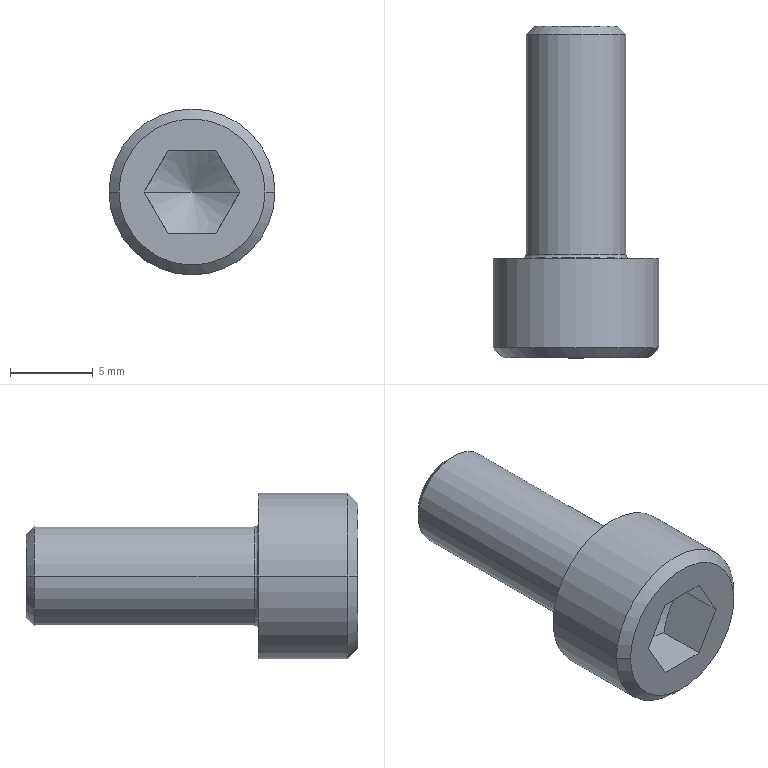Part | Creo | 1 solid | 23 faces | box 10 x 20 x 10 mm | volume 780.586 mm3 | plane 9 | cone 6 | cylinder 4 | torus 4 | commonest cylinder face diameters 6 x2 10 x2
STEP:
#1=CARTESIAN_POINT('',(0.,0.,0.));
#2=DIRECTION('',(0.,0.,1.));
#3=DIRECTION('',(1.,0.,0.));
#4=AXIS2_PLACEMENT_3D('',#1,#2,#3);
#5=CARTESIAN_POINT('',(-46.437,-246.,-26.767));
#6=VERTEX_POINT('',#5);
#7=CARTESIAN_POINT('',(-44.993,-246.,-29.267));
#8=VERTEX_POINT('',#7);
#9=CARTESIAN_POINT('',(-46.437,-246.,-26.767));
#10=CARTESIAN_POINT('',(-46.401,-245.979,-26.83));
#11=CARTESIAN_POINT('',(-46.329,-245.94,-26.953));
#12=CARTESIAN_POINT('',(-46.226,-245.891,-27.132));
#13=CARTESIAN_POINT('',(-46.124,-245.851,-27.308));
#14=CARTESIAN_POINT('',(-46.024,-245.819,-27.483));
#15=CARTESIAN_POINT('',(-45.922,-245.795,-27.659));
#16=CARTESIAN_POINT('',(-45.819,-245.78,-27.837));
#17=CARTESIAN_POINT('',(-45.715,-245.775,-28.017));
#18=CARTESIAN_POINT('',(-45.611,-245.78,-28.197));
#19=CARTESIAN_POINT('',(-45.508,-245.795,-28.375));
#20=CARTESIAN_POINT('',(-45.407,-245.819,-28.551));
#21=CARTESIAN_POINT('',(-45.306,-245.851,-28.726));
#22=CARTESIAN_POINT('',(-45.204,-245.891,-28.902));
#23=CARTESIAN_POINT('',(-45.101,-245.94,-29.081));
#24=CARTESIAN_POINT('',(-45.03,-245.979,-29.204));
#25=CARTESIAN_POINT('',(-44.993,-246.,-29.267));
#26=B_SPLINE_CURVE_WITH_KNOTS('',3,(#9,#10,#11,#12,#13,#14,#15,#16,#17,#18,#19,#20,#21,#22,#23,#24,#25),.UNSPECIFIED.,.F.,.F.,(4,1,1,1,1,1,1,1,1,1,1,1,1,1,4),(0.,0.07143,0.1429,0.2143,0.2857,0.3571,0.4286,0.5,0.5714,0.6429,0.7143,0.7857,0.8571,0.9286,1.),.UNSPECIFIED.);
#27=EDGE_CURVE('',#6,#8,#26,.T.);
#28=ORIENTED_EDGE('',*,*,#27,.F.);
#29=CARTESIAN_POINT('',(-43.55,-244.333,-26.767));
#30=VERTEX_POINT('',#29);
#31=CARTESIAN_POINT('',(-43.55,-244.333,-26.767));
#32=DIRECTION('',(-0.866,-0.5,0.));
#33=VECTOR('',#32,3.333);
#34=LINE('',#31,#33);
#35=EDGE_CURVE('',#30,#6,#34,.T.);
#36=ORIENTED_EDGE('',*,*,#35,.F.);
#37=CARTESIAN_POINT('',(-40.663,-246.,-26.767));
#38=VERTEX_POINT('',#37);
#39=CARTESIAN_POINT('',(-43.55,-244.333,-26.767));
#40=DIRECTION('',(0.866,-0.5,0.));
#41=VECTOR('',#40,3.333);
#42=LINE('',#39,#41);
#43=EDGE_CURVE('',#30,#38,#42,.T.);
#44=ORIENTED_EDGE('',*,*,#43,.T.);
#45=CARTESIAN_POINT('',(-42.107,-246.,-29.267));
#46=VERTEX_POINT('',#45);
#47=CARTESIAN_POINT('',(-42.107,-246.,-29.267));
#48=CARTESIAN_POINT('',(-42.07,-245.979,-29.204));
#49=CARTESIAN_POINT('',(-41.999,-245.94,-29.081));
#50=CARTESIAN_POINT('',(-41.896,-245.891,-28.902));
#51=CARTESIAN_POINT('',(-41.794,-245.851,-28.726));
#52=CARTESIAN_POINT('',(-41.693,-245.819,-28.551));
#53=CARTESIAN_POINT('',(-41.592,-245.795,-28.375));
#54=CARTESIAN_POINT('',(-41.489,-245.78,-28.197));
#55=CARTESIAN_POINT('',(-41.385,-245.775,-28.017));
#56=CARTESIAN_POINT('',(-41.281,-245.78,-27.837));
#57=CARTESIAN_POINT('',(-41.178,-245.795,-27.659));
#58=CARTESIAN_POINT('',(-41.076,-245.819,-27.483));
#59=CARTESIAN_POINT('',(-40.976,-245.851,-27.308));
#60=CARTESIAN_POINT('',(-40.874,-245.891,-27.132));
#61=CARTESIAN_POINT('',(-40.771,-245.94,-26.953));
#62=CARTESIAN_POINT('',(-40.699,-245.979,-26.83));
#63=CARTESIAN_POINT('',(-40.663,-246.,-26.767));
#64=B_SPLINE_CURVE_WITH_KNOTS('',3,(#47,#48,#49,#50,#51,#52,#53,#54,#55,#56,#57,#58,#59,#60,#61,#62,#63),.UNSPECIFIED.,.F.,.F.,(4,1,1,1,1,1,1,1,1,1,1,1,1,1,4),(0.,0.07143,0.1429,0.2143,0.2857,0.3571,0.4286,0.5,0.5714,0.6429,0.7143,0.7857,0.8571,0.9286,1.),.UNSPECIFIED.);
#65=EDGE_CURVE('',#46,#38,#64,.T.);
#66=ORIENTED_EDGE('',*,*,#65,.F.);
#67=CARTESIAN_POINT('',(-44.993,-246.,-29.267));
#68=CARTESIAN_POINT('',(-44.921,-245.979,-29.267));
#69=CARTESIAN_POINT('',(-44.778,-245.94,-29.267));
#70=CARTESIAN_POINT('',(-44.572,-245.891,-29.267));
#71=CARTESIAN_POINT('',(-44.37,-245.851,-29.267));
#72=CARTESIAN_POINT('',(-44.168,-245.819,-29.267));
#73=CARTESIAN_POINT('',(-43.964,-245.795,-29.267));
#74=CARTESIAN_POINT('',(-43.758,-245.78,-29.267));
#75=CARTESIAN_POINT('',(-43.55,-245.775,-29.267));
#76=CARTESIAN_POINT('',(-43.342,-245.78,-29.267));
#77=CARTESIAN_POINT('',(-43.136,-245.795,-29.267));
#78=CARTESIAN_POINT('',(-42.932,-245.819,-29.267));
#79=CARTESIAN_POINT('',(-42.73,-245.851,-29.267));
#80=CARTESIAN_POINT('',(-42.528,-245.891,-29.267));
#81=CARTESIAN_POINT('',(-42.322,-245.94,-29.267));
#82=CARTESIAN_POINT('',(-42.179,-245.979,-29.267));
#83=CARTESIAN_POINT('',(-42.107,-246.,-29.267));
#84=B_SPLINE_CURVE_WITH_KNOTS('',3,(#67,#68,#69,#70,#71,#72,#73,#74,#75,#76,#77,#78,#79,#80,#81,#82,#83),.UNSPECIFIED.,.F.,.F.,(4,1,1,1,1,1,1,1,1,1,1,1,1,1,4),(0.,0.07143,0.1429,0.2143,0.2857,0.3571,0.4286,0.5,0.5714,0.6429,0.7143,0.7857,0.8571,0.9286,1.),.UNSPECIFIED.);
#85=EDGE_CURVE('',#8,#46,#84,.T.);
#86=ORIENTED_EDGE('',*,*,#85,.F.);
#87=EDGE_LOOP('',(#28,#36,#44,#66,#86));
#88=FACE_OUTER_BOUND('',#87,.F.);
#89=CARTESIAN_POINT('',(-43.55,-245.183,-26.767));
#90=DIRECTION('',(0.,-1.,0.));
#91=DIRECTION('',(-1.,0.,0.));
#92=AXIS2_PLACEMENT_3D('',#89,#90,#91);
#93=CONICAL_SURFACE('',#92,1.472,60.);
#94=ADVANCED_FACE('',(#88),#93,.F.);
#95=CARTESIAN_POINT('',(-44.993,-249.,-29.267));
#96=VERTEX_POINT('',#95);
#97=CARTESIAN_POINT('',(-46.437,-249.,-26.767));
#98=VERTEX_POINT('',#97);
#99=CARTESIAN_POINT('',(-44.993,-249.,-29.267));
#100=DIRECTION('',(-0.5,0.,0.866));
#101=VECTOR('',#100,2.887);
#102=LINE('',#99,#101);
#103=EDGE_CURVE('',#96,#98,#102,.T.);
#104=ORIENTED_EDGE('',*,*,#103,.T.);
#105=CARTESIAN_POINT('',(-46.437,-249.,-26.767));
#106=DIRECTION('',(0.,1.,0.));
#107=VECTOR('',#106,3.);
#108=LINE('',#105,#107);
#109=EDGE_CURVE('',#98,#6,#108,.T.);
#110=ORIENTED_EDGE('',*,*,#109,.T.);
#111=ORIENTED_EDGE('',*,*,#27,.T.);
#112=CARTESIAN_POINT('',(-44.993,-249.,-29.267));
#113=DIRECTION('',(0.,1.,0.));
#114=VECTOR('',#113,3.);
#115=LINE('',#112,#114);
#116=EDGE_CURVE('',#96,#8,#115,.T.);
#117=ORIENTED_EDGE('',*,*,#116,.F.);
#118=EDGE_LOOP('',(#104,#110,#111,#117));
#119=FACE_OUTER_BOUND('',#118,.F.);
#120=CARTESIAN_POINT('',(-44.993,-246.,-29.267));
#121=DIRECTION('',(0.866,0.,0.5));
#122=DIRECTION('',(-0.5,0.,0.866));
#123=AXIS2_PLACEMENT_3D('',#120,#121,#122);
#124=PLANE('',#123);
#125=ADVANCED_FACE('',(#119),#124,.T.);
#126=CARTESIAN_POINT('',(-47.95,-249.,-26.767));
#127=VERTEX_POINT('',#126);
#128=CARTESIAN_POINT('',(-39.15,-249.,-26.767));
#129=VERTEX_POINT('',#128);
#130=CARTESIAN_POINT('',(-43.55,-249.,-26.767));
#131=DIRECTION('',(0.,-1.,0.));
#132=DIRECTION('',(-1.,0.,0.));
#133=AXIS2_PLACEMENT_3D('',#130,#131,#132);
#134=CIRCLE('',#133,4.4);
#135=EDGE_CURVE('',#127,#129,#134,.T.);
#136=ORIENTED_EDGE('',*,*,#135,.F.);
#137=CARTESIAN_POINT('',(-43.55,-249.,-26.767));
#138=DIRECTION('',(0.,-1.,0.));
#139=DIRECTION('',(1.,0.,0.));
#140=AXIS2_PLACEMENT_3D('',#137,#138,#139);
#141=CIRCLE('',#140,4.4);
#142=EDGE_CURVE('',#129,#127,#141,.T.);
#143=ORIENTED_EDGE('',*,*,#142,.F.);
#144=EDGE_LOOP('',(#136,#143));
#145=FACE_OUTER_BOUND('',#144,.F.);
#146=CARTESIAN_POINT('',(-44.993,-249.,-24.267));
#147=VERTEX_POINT('',#146);
#148=CARTESIAN_POINT('',(-46.437,-249.,-26.767));
#149=DIRECTION('',(0.5,0.,0.866));
#150=VECTOR('',#149,2.887);
#151=LINE('',#148,#150);
#152=EDGE_CURVE('',#98,#147,#151,.T.);
#153=ORIENTED_EDGE('',*,*,#152,.F.);
#154=ORIENTED_EDGE('',*,*,#103,.F.);
#155=CARTESIAN_POINT('',(-42.107,-249.,-29.267));
#156=VERTEX_POINT('',#155);
#157=CARTESIAN_POINT('',(-44.993,-249.,-29.267));
#158=DIRECTION('',(1.,0.,0.));
#159=VECTOR('',#158,2.887);
#160=LINE('',#157,#159);
#161=EDGE_CURVE('',#96,#156,#160,.T.);
#162=ORIENTED_EDGE('',*,*,#161,.T.);
#163=CARTESIAN_POINT('',(-40.663,-249.,-26.767));
#164=VERTEX_POINT('',#163);
#165=CARTESIAN_POINT('',(-40.663,-249.,-26.767));
#166=DIRECTION('',(-0.5,0.,-0.866));
#167=VECTOR('',#166,2.887);
#168=LINE('',#165,#167);
#169=EDGE_CURVE('',#164,#156,#168,.T.);
#170=ORIENTED_EDGE('',*,*,#169,.F.);
#171=CARTESIAN_POINT('',(-42.107,-249.,-24.267));
#172=VERTEX_POINT('',#171);
#173=CARTESIAN_POINT('',(-42.107,-249.,-24.267));
#174=DIRECTION('',(0.5,0.,-0.866));
#175=VECTOR('',#174,2.887);
#176=LINE('',#173,#175);
#177=EDGE_CURVE('',#172,#164,#176,.T.);
#178=ORIENTED_EDGE('',*,*,#177,.F.);
#179=CARTESIAN_POINT('',(-42.107,-249.,-24.267));
#180=DIRECTION('',(-1.,0.,0.));
#181=VECTOR('',#180,2.887);
#182=LINE('',#179,#181);
#183=EDGE_CURVE('',#172,#147,#182,.T.);
#184=ORIENTED_EDGE('',*,*,#183,.T.);
#185=EDGE_LOOP('',(#153,#154,#162,#170,#178,#184));
#186=FACE_BOUND('',#185,.F.);
#187=CARTESIAN_POINT('',(-43.55,-249.,-26.767));
#188=DIRECTION('',(0.,-1.,0.));
#189=DIRECTION('',(-1.,0.,0.));
#190=AXIS2_PLACEMENT_3D('',#187,#188,#189);
#191=PLANE('',#190);
#192=ADVANCED_FACE('',(#145,#186),#191,.T.);
#193=CARTESIAN_POINT('',(-48.55,-248.4,-26.767));
#194=VERTEX_POINT('',#193);
#195=CARTESIAN_POINT('',(-38.55,-248.4,-26.767));
#196=VERTEX_POINT('',#195);
#197=CARTESIAN_POINT('',(-43.55,-248.4,-26.767));
#198=DIRECTION('',(0.,-1.,0.));
#199=DIRECTION('',(-1.,0.,0.));
#200=AXIS2_PLACEMENT_3D('',#197,#198,#199);
#201=CIRCLE('',#200,5.);
#202=EDGE_CURVE('',#194,#196,#201,.T.);
#203=ORIENTED_EDGE('',*,*,#202,.F.);
#204=CARTESIAN_POINT('',(-47.95,-249.,-26.767));
#205=DIRECTION('',(-0.7071,0.7071,0.));
#206=VECTOR('',#205,0.8485);
#207=LINE('',#204,#206);
#208=EDGE_CURVE('',#127,#194,#207,.T.);
#209=ORIENTED_EDGE('',*,*,#208,.F.);
#210=ORIENTED_EDGE('',*,*,#135,.T.);
#211=CARTESIAN_POINT('',(-39.15,-249.,-26.767));
#212=DIRECTION('',(0.7071,0.7071,0.));
#213=VECTOR('',#212,0.8485);
#214=LINE('',#211,#213);
#215=EDGE_CURVE('',#129,#196,#214,.T.);
#216=ORIENTED_EDGE('',*,*,#215,.T.);
#217=EDGE_LOOP('',(#203,#209,#210,#216));
#218=FACE_OUTER_BOUND('',#217,.F.);
#219=CARTESIAN_POINT('',(-43.55,-248.7,-26.767));
#220=DIRECTION('',(0.,1.,0.));
#221=DIRECTION('',(1.,0.,0.));
#222=AXIS2_PLACEMENT_3D('',#219,#220,#221);
#223=CONICAL_SURFACE('',#222,4.7,45.);
#224=ADVANCED_FACE('',(#218),#223,.T.);
#225=ORIENTED_EDGE('',*,*,#202,.T.);
#226=CARTESIAN_POINT('',(-38.55,-243.,-26.767));
#227=VERTEX_POINT('',#226);
#228=CARTESIAN_POINT('',(-38.55,-243.,-26.767));
#229=DIRECTION('',(0.,-1.,0.));
#230=VECTOR('',#229,5.4);
#231=LINE('',#228,#230);
#232=EDGE_CURVE('',#227,#196,#231,.T.);
#233=ORIENTED_EDGE('',*,*,#232,.F.);
#234=CARTESIAN_POINT('',(-48.55,-243.,-26.767));
#235=VERTEX_POINT('',#234);
#236=CARTESIAN_POINT('',(-43.55,-243.,-26.767));
#237=DIRECTION('',(0.,1.,0.));
#238=DIRECTION('',(1.,0.,0.));
#239=AXIS2_PLACEMENT_3D('',#236,#237,#238);
#240=CIRCLE('',#239,5.);
#241=EDGE_CURVE('',#227,#235,#240,.T.);
#242=ORIENTED_EDGE('',*,*,#241,.T.);
#243=CARTESIAN_POINT('',(-48.55,-243.,-26.767));
#244=DIRECTION('',(0.,-1.,0.));
#245=VECTOR('',#244,5.4);
#246=LINE('',#243,#245);
#247=EDGE_CURVE('',#235,#194,#246,.T.);
#248=ORIENTED_EDGE('',*,*,#247,.T.);
#249=EDGE_LOOP('',(#225,#233,#242,#248));
#250=FACE_OUTER_BOUND('',#249,.F.);
#251=CARTESIAN_POINT('',(-43.55,-243.,-26.767));
#252=DIRECTION('',(0.,-1.,0.));
#253=DIRECTION('',(-1.,0.,0.));
#254=AXIS2_PLACEMENT_3D('',#251,#252,#253);
#255=CYLINDRICAL_SURFACE('',#254,5.);
#256=ADVANCED_FACE('',(#250),#255,.T.);
#257=CARTESIAN_POINT('',(-43.55,-248.4,-26.767));
#258=DIRECTION('',(0.,-1.,0.));
#259=DIRECTION('',(1.,0.,0.));
#260=AXIS2_PLACEMENT_3D('',#257,#258,#259);
#261=CIRCLE('',#260,5.);
#262=EDGE_CURVE('',#196,#194,#261,.T.);
#263=ORIENTED_EDGE('',*,*,#262,.T.);
#264=ORIENTED_EDGE('',*,*,#247,.F.);
#265=CARTESIAN_POINT('',(-43.55,-243.,-26.767));
#266=DIRECTION('',(0.,1.,0.));
#267=DIRECTION('',(-1.,0.,0.));
#268=AXIS2_PLACEMENT_3D('',#265,#266,#267);
#269=CIRCLE('',#268,5.);
#270=EDGE_CURVE('',#235,#227,#269,.T.);
#271=ORIENTED_EDGE('',*,*,#270,.T.);
#272=ORIENTED_EDGE('',*,*,#232,.T.);
#273=EDGE_LOOP('',(#263,#264,#271,#272));
#274=FACE_OUTER_BOUND('',#273,.F.);
#275=CARTESIAN_POINT('',(-43.55,-243.,-26.767));
#276=DIRECTION('',(0.,-1.,0.));
#277=DIRECTION('',(-1.,0.,0.));
#278=AXIS2_PLACEMENT_3D('',#275,#276,#277);
#279=CYLINDRICAL_SURFACE('',#278,5.);
#280=ADVANCED_FACE('',(#274),#279,.T.);
#281=ORIENTED_EDGE('',*,*,#262,.F.);
#282=ORIENTED_EDGE('',*,*,#215,.F.);
#283=ORIENTED_EDGE('',*,*,#142,.T.);
#284=ORIENTED_EDGE('',*,*,#208,.T.);
#285=EDGE_LOOP('',(#281,#282,#283,#284));
#286=FACE_OUTER_BOUND('',#285,.F.);
#287=CARTESIAN_POINT('',(-43.55,-248.7,-26.767));
#288=DIRECTION('',(0.,1.,0.));
#289=DIRECTION('',(1.,0.,0.));
#290=AXIS2_PLACEMENT_3D('',#287,#288,#289);
#291=CONICAL_SURFACE('',#290,4.7,45.);
#292=ADVANCED_FACE('',(#286),#291,.T.);
#293=ORIENTED_EDGE('',*,*,#270,.F.);
#294=ORIENTED_EDGE('',*,*,#241,.F.);
#295=EDGE_LOOP('',(#293,#294));
#296=FACE_OUTER_BOUND('',#295,.F.);
#297=CARTESIAN_POINT('',(-46.8,-243.,-26.767));
#298=VERTEX_POINT('',#297);
#299=CARTESIAN_POINT('',(-40.3,-243.,-26.767));
#300=VERTEX_POINT('',#299);
#301=CARTESIAN_POINT('',(-43.55,-243.,-26.767));
#302=DIRECTION('',(0.,-1.,0.));
#303=DIRECTION('',(-1.,0.,0.));
#304=AXIS2_PLACEMENT_3D('',#301,#302,#303);
#305=CIRCLE('',#304,3.25);
#306=EDGE_CURVE('',#298,#300,#305,.T.);
#307=ORIENTED_EDGE('',*,*,#306,.F.);
#308=CARTESIAN_POINT('',(-43.55,-243.,-26.767));
#309=DIRECTION('',(0.,-1.,0.));
#310=DIRECTION('',(1.,0.,0.));
#311=AXIS2_PLACEMENT_3D('',#308,#309,#310);
#312=CIRCLE('',#311,3.25);
#313=EDGE_CURVE('',#300,#298,#312,.T.);
#314=ORIENTED_EDGE('',*,*,#313,.F.);
#315=EDGE_LOOP('',(#307,#314));
#316=FACE_BOUND('',#315,.F.);
#317=CARTESIAN_POINT('',(-43.55,-243.,-26.767));
#318=DIRECTION('',(0.,-1.,0.));
#319=DIRECTION('',(-1.,0.,0.));
#320=AXIS2_PLACEMENT_3D('',#317,#318,#319);
#321=PLANE('',#320);
#322=ADVANCED_FACE('',(#296,#316),#321,.F.);
#323=ORIENTED_EDGE('',*,*,#306,.T.);
#324=CARTESIAN_POINT('',(-40.477,-242.927,-26.767));
#325=VERTEX_POINT('',#324);
#326=CARTESIAN_POINT('',(-40.3,-242.75,-26.767));
#327=DIRECTION('',(0.,0.,-1.));
#328=DIRECTION('',(0.,-1.,0.));
#329=AXIS2_PLACEMENT_3D('',#326,#327,#328);
#330=CIRCLE('',#329,0.25);
#331=EDGE_CURVE('',#300,#325,#330,.T.);
#332=ORIENTED_EDGE('',*,*,#331,.T.);
#333=CARTESIAN_POINT('',(-46.623,-242.927,-26.767));
#334=VERTEX_POINT('',#333);
#335=CARTESIAN_POINT('',(-43.55,-242.927,-26.767));
#336=DIRECTION('',(0.,-1.,0.));
#337=DIRECTION('',(-1.,0.,0.));
#338=AXIS2_PLACEMENT_3D('',#335,#336,#337);
#339=CIRCLE('',#338,3.073);
#340=EDGE_CURVE('',#334,#325,#339,.T.);
#341=ORIENTED_EDGE('',*,*,#340,.F.);
#342=CARTESIAN_POINT('',(-46.8,-242.75,-26.767));
#343=DIRECTION('',(0.,0.,1.));
#344=DIRECTION('',(0.,-1.,0.));
#345=AXIS2_PLACEMENT_3D('',#342,#343,#344);
#346=CIRCLE('',#345,0.25);
#347=EDGE_CURVE('',#298,#334,#346,.T.);
#348=ORIENTED_EDGE('',*,*,#347,.F.);
#349=EDGE_LOOP('',(#323,#332,#341,#348));
#350=FACE_OUTER_BOUND('',#349,.F.);
#351=CARTESIAN_POINT('',(-43.55,-242.75,-26.767));
#352=DIRECTION('',(0.,-1.,0.));
#353=DIRECTION('',(-1.,0.,0.));
#354=AXIS2_PLACEMENT_3D('',#351,#352,#353);
#355=TOROIDAL_SURFACE('',#354,3.25,0.25);
#356=ADVANCED_FACE('',(#350),#355,.F.);
#357=ORIENTED_EDGE('',*,*,#313,.T.);
#358=ORIENTED_EDGE('',*,*,#347,.T.);
#359=CARTESIAN_POINT('',(-43.55,-242.927,-26.767));
#360=DIRECTION('',(0.,-1.,0.));
#361=DIRECTION('',(1.,0.,0.));
#362=AXIS2_PLACEMENT_3D('',#359,#360,#361);
#363=CIRCLE('',#362,3.073);
#364=EDGE_CURVE('',#325,#334,#363,.T.);
#365=ORIENTED_EDGE('',*,*,#364,.F.);
#366=ORIENTED_EDGE('',*,*,#331,.F.);
#367=EDGE_LOOP('',(#357,#358,#365,#366));
#368=FACE_OUTER_BOUND('',#367,.F.);
#369=CARTESIAN_POINT('',(-43.55,-242.75,-26.767));
#370=DIRECTION('',(0.,-1.,0.));
#371=DIRECTION('',(-1.,0.,0.));
#372=AXIS2_PLACEMENT_3D('',#369,#370,#371);
#373=TOROIDAL_SURFACE('',#372,3.25,0.25);
#374=ADVANCED_FACE('',(#368),#373,.F.);
#375=CARTESIAN_POINT('',(-40.55,-242.75,-26.767));
#376=VERTEX_POINT('',#375);
#377=CARTESIAN_POINT('',(-46.55,-242.75,-26.767));
#378=VERTEX_POINT('',#377);
#379=CARTESIAN_POINT('',(-43.55,-242.75,-26.767));
#380=DIRECTION('',(0.,-1.,0.));
#381=DIRECTION('',(1.,0.,0.));
#382=AXIS2_PLACEMENT_3D('',#379,#380,#381);
#383=CIRCLE('',#382,3.);
#384=EDGE_CURVE('',#376,#378,#383,.T.);
#385=ORIENTED_EDGE('',*,*,#384,.F.);
#386=CARTESIAN_POINT('',(-40.3,-242.75,-26.767));
#387=DIRECTION('',(0.,0.,-1.));
#388=DIRECTION('',(-0.7071,-0.7071,0.));
#389=AXIS2_PLACEMENT_3D('',#386,#387,#388);
#390=CIRCLE('',#389,0.25);
#391=EDGE_CURVE('',#325,#376,#390,.T.);
#392=ORIENTED_EDGE('',*,*,#391,.F.);
#393=ORIENTED_EDGE('',*,*,#364,.T.);
#394=CARTESIAN_POINT('',(-46.8,-242.75,-26.767));
#395=DIRECTION('',(0.,0.,1.));
#396=DIRECTION('',(0.7071,-0.7071,0.));
#397=AXIS2_PLACEMENT_3D('',#394,#395,#396);
#398=CIRCLE('',#397,0.25);
#399=EDGE_CURVE('',#334,#378,#398,.T.);
#400=ORIENTED_EDGE('',*,*,#399,.T.);
#401=EDGE_LOOP('',(#385,#392,#393,#400));
#402=FACE_OUTER_BOUND('',#401,.F.);
#403=CARTESIAN_POINT('',(-43.55,-242.75,-26.767));
#404=DIRECTION('',(0.,-1.,0.));
#405=DIRECTION('',(-1.,0.,0.));
#406=AXIS2_PLACEMENT_3D('',#403,#404,#405);
#407=TOROIDAL_SURFACE('',#406,3.25,0.25);
#408=ADVANCED_FACE('',(#402),#407,.F.);
#409=CARTESIAN_POINT('',(-46.55,-229.5,-26.767));
#410=VERTEX_POINT('',#409);
#411=CARTESIAN_POINT('',(-40.55,-229.5,-26.767));
#412=VERTEX_POINT('',#411);
#413=CARTESIAN_POINT('',(-43.55,-229.5,-26.767));
#414=DIRECTION('',(0.,1.,0.));
#415=DIRECTION('',(-1.,0.,0.));
#416=AXIS2_PLACEMENT_3D('',#413,#414,#415);
#417=CIRCLE('',#416,3.);
#418=EDGE_CURVE('',#410,#412,#417,.T.);
#419=ORIENTED_EDGE('',*,*,#418,.T.);
#420=CARTESIAN_POINT('',(-40.55,-229.5,-26.767));
#421=DIRECTION('',(0.,-1.,0.));
#422=VECTOR('',#421,13.25);
#423=LINE('',#420,#422);
#424=EDGE_CURVE('',#412,#376,#423,.T.);
#425=ORIENTED_EDGE('',*,*,#424,.T.);
#426=ORIENTED_EDGE('',*,*,#384,.T.);
#427=CARTESIAN_POINT('',(-46.55,-229.5,-26.767));
#428=DIRECTION('',(0.,-1.,0.));
#429=VECTOR('',#428,13.25);
#430=LINE('',#427,#429);
#431=EDGE_CURVE('',#410,#378,#430,.T.);
#432=ORIENTED_EDGE('',*,*,#431,.F.);
#433=EDGE_LOOP('',(#419,#425,#426,#432));
#434=FACE_OUTER_BOUND('',#433,.F.);
#435=CARTESIAN_POINT('',(-43.55,-229.,-26.767));
#436=DIRECTION('',(0.,-1.,0.));
#437=DIRECTION('',(-1.,0.,0.));
#438=AXIS2_PLACEMENT_3D('',#435,#436,#437);
#439=CYLINDRICAL_SURFACE('',#438,3.);
#440=ADVANCED_FACE('',(#434),#439,.T.);
#441=CARTESIAN_POINT('',(-46.05,-229.,-26.767));
#442=VERTEX_POINT('',#441);
#443=CARTESIAN_POINT('',(-41.05,-229.,-26.767));
#444=VERTEX_POINT('',#443);
#445=CARTESIAN_POINT('',(-43.55,-229.,-26.767));
#446=DIRECTION('',(0.,1.,0.));
#447=DIRECTION('',(-1.,0.,0.));
#448=AXIS2_PLACEMENT_3D('',#445,#446,#447);
#449=CIRCLE('',#448,2.5);
#450=EDGE_CURVE('',#442,#444,#449,.T.);
#451=ORIENTED_EDGE('',*,*,#450,.T.);
#452=CARTESIAN_POINT('',(-41.05,-229.,-26.767));
#453=DIRECTION('',(0.7071,-0.7071,0.));
#454=VECTOR('',#453,0.7071);
#455=LINE('',#452,#454);
#456=EDGE_CURVE('',#444,#412,#455,.T.);
#457=ORIENTED_EDGE('',*,*,#456,.T.);
#458=ORIENTED_EDGE('',*,*,#418,.F.);
#459=CARTESIAN_POINT('',(-46.05,-229.,-26.767));
#460=DIRECTION('',(-0.7071,-0.7071,0.));
#461=VECTOR('',#460,0.7071);
#462=LINE('',#459,#461);
#463=EDGE_CURVE('',#442,#410,#462,.T.);
#464=ORIENTED_EDGE('',*,*,#463,.F.);
#465=EDGE_LOOP('',(#451,#457,#458,#464));
#466=FACE_OUTER_BOUND('',#465,.F.);
#467=CARTESIAN_POINT('',(-43.55,-229.25,-26.767));
#468=DIRECTION('',(0.,-1.,0.));
#469=DIRECTION('',(-1.,0.,0.));
#470=AXIS2_PLACEMENT_3D('',#467,#468,#469);
#471=CONICAL_SURFACE('',#470,2.75,45.);
#472=ADVANCED_FACE('',(#466),#471,.T.);
#473=ORIENTED_EDGE('',*,*,#450,.F.);
#474=CARTESIAN_POINT('',(-43.55,-229.,-26.767));
#475=DIRECTION('',(0.,1.,0.));
#476=DIRECTION('',(1.,0.,0.));
#477=AXIS2_PLACEMENT_3D('',#474,#475,#476);
#478=CIRCLE('',#477,2.5);
#479=EDGE_CURVE('',#444,#442,#478,.T.);
#480=ORIENTED_EDGE('',*,*,#479,.F.);
#481=EDGE_LOOP('',(#473,#480));
#482=FACE_OUTER_BOUND('',#481,.F.);
#483=CARTESIAN_POINT('',(-43.55,-229.,-26.767));
#484=DIRECTION('',(0.,-1.,0.));
#485=DIRECTION('',(-1.,0.,0.));
#486=AXIS2_PLACEMENT_3D('',#483,#484,#485);
#487=PLANE('',#486);
#488=ADVANCED_FACE('',(#482),#487,.F.);
#489=ORIENTED_EDGE('',*,*,#479,.T.);
#490=ORIENTED_EDGE('',*,*,#463,.T.);
#491=CARTESIAN_POINT('',(-43.55,-229.5,-26.767));
#492=DIRECTION('',(0.,1.,0.));
#493=DIRECTION('',(1.,0.,0.));
#494=AXIS2_PLACEMENT_3D('',#491,#492,#493);
#495=CIRCLE('',#494,3.);
#496=EDGE_CURVE('',#412,#410,#495,.T.);
#497=ORIENTED_EDGE('',*,*,#496,.F.);
#498=ORIENTED_EDGE('',*,*,#456,.F.);
#499=EDGE_LOOP('',(#489,#490,#497,#498));
#500=FACE_OUTER_BOUND('',#499,.F.);
#501=CARTESIAN_POINT('',(-43.55,-229.25,-26.767));
#502=DIRECTION('',(0.,-1.,0.));
#503=DIRECTION('',(-1.,0.,0.));
#504=AXIS2_PLACEMENT_3D('',#501,#502,#503);
#505=CONICAL_SURFACE('',#504,2.75,45.);
#506=ADVANCED_FACE('',(#500),#505,.T.);
#507=ORIENTED_EDGE('',*,*,#496,.T.);
#508=ORIENTED_EDGE('',*,*,#431,.T.);
#509=CARTESIAN_POINT('',(-43.55,-242.75,-26.767));
#510=DIRECTION('',(0.,-1.,0.));
#511=DIRECTION('',(-1.,0.,0.));
#512=AXIS2_PLACEMENT_3D('',#509,#510,#511);
#513=CIRCLE('',#512,3.);
#514=EDGE_CURVE('',#378,#376,#513,.T.);
#515=ORIENTED_EDGE('',*,*,#514,.T.);
#516=ORIENTED_EDGE('',*,*,#424,.F.);
#517=EDGE_LOOP('',(#507,#508,#515,#516));
#518=FACE_OUTER_BOUND('',#517,.F.);
#519=CARTESIAN_POINT('',(-43.55,-229.,-26.767));
#520=DIRECTION('',(0.,-1.,0.));
#521=DIRECTION('',(-1.,0.,0.));
#522=AXIS2_PLACEMENT_3D('',#519,#520,#521);
#523=CYLINDRICAL_SURFACE('',#522,3.);
#524=ADVANCED_FACE('',(#518),#523,.T.);
#525=ORIENTED_EDGE('',*,*,#514,.F.);
#526=ORIENTED_EDGE('',*,*,#399,.F.);
#527=ORIENTED_EDGE('',*,*,#340,.T.);
#528=ORIENTED_EDGE('',*,*,#391,.T.);
#529=EDGE_LOOP('',(#525,#526,#527,#528));
#530=FACE_OUTER_BOUND('',#529,.F.);
#531=CARTESIAN_POINT('',(-43.55,-242.75,-26.767));
#532=DIRECTION('',(0.,-1.,0.));
#533=DIRECTION('',(-1.,0.,0.));
#534=AXIS2_PLACEMENT_3D('',#531,#532,#533);
#535=TOROIDAL_SURFACE('',#534,3.25,0.25);
#536=ADVANCED_FACE('',(#530),#535,.F.);
#537=ORIENTED_EDGE('',*,*,#152,.T.);
#538=CARTESIAN_POINT('',(-44.993,-246.,-24.267));
#539=VERTEX_POINT('',#538);
#540=CARTESIAN_POINT('',(-44.993,-249.,-24.267));
#541=DIRECTION('',(0.,1.,0.));
#542=VECTOR('',#541,3.);
#543=LINE('',#540,#542);
#544=EDGE_CURVE('',#147,#539,#543,.T.);
#545=ORIENTED_EDGE('',*,*,#544,.T.);
#546=CARTESIAN_POINT('',(-44.993,-246.,-24.267));
#547=CARTESIAN_POINT('',(-45.03,-245.979,-24.33));
#548=CARTESIAN_POINT('',(-45.101,-245.94,-24.453));
#549=CARTESIAN_POINT('',(-45.204,-245.891,-24.632));
#550=CARTESIAN_POINT('',(-45.306,-245.851,-24.808));
#551=CARTESIAN_POINT('',(-45.407,-245.819,-24.983));
#552=CARTESIAN_POINT('',(-45.508,-245.795,-25.159));
#553=CARTESIAN_POINT('',(-45.611,-245.78,-25.337));
#554=CARTESIAN_POINT('',(-45.715,-245.775,-25.517));
#555=CARTESIAN_POINT('',(-45.819,-245.78,-25.697));
#556=CARTESIAN_POINT('',(-45.922,-245.795,-25.875));
#557=CARTESIAN_POINT('',(-46.024,-245.819,-26.051));
#558=CARTESIAN_POINT('',(-46.124,-245.851,-26.226));
#559=CARTESIAN_POINT('',(-46.226,-245.891,-26.402));
#560=CARTESIAN_POINT('',(-46.329,-245.94,-26.581));
#561=CARTESIAN_POINT('',(-46.401,-245.979,-26.704));
#562=CARTESIAN_POINT('',(-46.437,-246.,-26.767));
#563=B_SPLINE_CURVE_WITH_KNOTS('',3,(#546,#547,#548,#549,#550,#551,#552,#553,#554,#555,#556,#557,#558,#559,#560,#561,#562),.UNSPECIFIED.,.F.,.F.,(4,1,1,1,1,1,1,1,1,1,1,1,1,1,4),(0.,0.07143,0.1429,0.2143,0.2857,0.3571,0.4286,0.5,0.5714,0.6429,0.7143,0.7857,0.8571,0.9286,1.),.UNSPECIFIED.);
#564=EDGE_CURVE('',#539,#6,#563,.T.);
#565=ORIENTED_EDGE('',*,*,#564,.T.);
#566=ORIENTED_EDGE('',*,*,#109,.F.);
#567=EDGE_LOOP('',(#537,#545,#565,#566));
#568=FACE_OUTER_BOUND('',#567,.F.);
#569=CARTESIAN_POINT('',(-46.437,-246.,-26.767));
#570=DIRECTION('',(0.866,0.,-0.5));
#571=DIRECTION('',(0.5,0.,0.866));
#572=AXIS2_PLACEMENT_3D('',#569,#570,#571);
#573=PLANE('',#572);
#574=ADVANCED_FACE('',(#568),#573,.T.);
#575=ORIENTED_EDGE('',*,*,#183,.F.);
#576=CARTESIAN_POINT('',(-42.107,-246.,-24.267));
#577=VERTEX_POINT('',#576);
#578=CARTESIAN_POINT('',(-42.107,-249.,-24.267));
#579=DIRECTION('',(0.,1.,0.));
#580=VECTOR('',#579,3.);
#581=LINE('',#578,#580);
#582=EDGE_CURVE('',#172,#577,#581,.T.);
#583=ORIENTED_EDGE('',*,*,#582,.T.);
#584=CARTESIAN_POINT('',(-42.107,-246.,-24.267));
#585=CARTESIAN_POINT('',(-42.179,-245.979,-24.267));
#586=CARTESIAN_POINT('',(-42.322,-245.94,-24.267));
#587=CARTESIAN_POINT('',(-42.528,-245.891,-24.267));
#588=CARTESIAN_POINT('',(-42.73,-245.851,-24.267));
#589=CARTESIAN_POINT('',(-42.932,-245.819,-24.267));
#590=CARTESIAN_POINT('',(-43.136,-245.795,-24.267));
#591=CARTESIAN_POINT('',(-43.342,-245.78,-24.267));
#592=CARTESIAN_POINT('',(-43.55,-245.775,-24.267));
#593=CARTESIAN_POINT('',(-43.758,-245.78,-24.267));
#594=CARTESIAN_POINT('',(-43.964,-245.795,-24.267));
#595=CARTESIAN_POINT('',(-44.168,-245.819,-24.267));
#596=CARTESIAN_POINT('',(-44.37,-245.851,-24.267));
#597=CARTESIAN_POINT('',(-44.572,-245.891,-24.267));
#598=CARTESIAN_POINT('',(-44.778,-245.94,-24.267));
#599=CARTESIAN_POINT('',(-44.921,-245.979,-24.267));
#600=CARTESIAN_POINT('',(-44.993,-246.,-24.267));
#601=B_SPLINE_CURVE_WITH_KNOTS('',3,(#584,#585,#586,#587,#588,#589,#590,#591,#592,#593,#594,#595,#596,#597,#598,#599,#600),.UNSPECIFIED.,.F.,.F.,(4,1,1,1,1,1,1,1,1,1,1,1,1,1,4),(0.,0.07143,0.1429,0.2143,0.2857,0.3571,0.4286,0.5,0.5714,0.6429,0.7143,0.7857,0.8571,0.9286,1.),.UNSPECIFIED.);
#602=EDGE_CURVE('',#577,#539,#601,.T.);
#603=ORIENTED_EDGE('',*,*,#602,.T.);
#604=ORIENTED_EDGE('',*,*,#544,.F.);
#605=EDGE_LOOP('',(#575,#583,#603,#604));
#606=FACE_OUTER_BOUND('',#605,.F.);
#607=CARTESIAN_POINT('',(-44.993,-246.,-24.267));
#608=DIRECTION('',(0.,0.,-1.));
#609=DIRECTION('',(0.,-1.,0.));
#610=AXIS2_PLACEMENT_3D('',#607,#608,#609);
#611=PLANE('',#610);
#612=ADVANCED_FACE('',(#606),#611,.T.);
#613=ORIENTED_EDGE('',*,*,#177,.T.);
#614=CARTESIAN_POINT('',(-40.663,-249.,-26.767));
#615=DIRECTION('',(0.,1.,0.));
#616=VECTOR('',#615,3.);
#617=LINE('',#614,#616);
#618=EDGE_CURVE('',#164,#38,#617,.T.);
#619=ORIENTED_EDGE('',*,*,#618,.T.);
#620=CARTESIAN_POINT('',(-40.663,-246.,-26.767));
#621=CARTESIAN_POINT('',(-40.699,-245.979,-26.704));
#622=CARTESIAN_POINT('',(-40.771,-245.94,-26.581));
#623=CARTESIAN_POINT('',(-40.874,-245.891,-26.402));
#624=CARTESIAN_POINT('',(-40.976,-245.851,-26.226));
#625=CARTESIAN_POINT('',(-41.076,-245.819,-26.051));
#626=CARTESIAN_POINT('',(-41.178,-245.795,-25.875));
#627=CARTESIAN_POINT('',(-41.281,-245.78,-25.697));
#628=CARTESIAN_POINT('',(-41.385,-245.775,-25.517));
#629=CARTESIAN_POINT('',(-41.489,-245.78,-25.337));
#630=CARTESIAN_POINT('',(-41.592,-245.795,-25.159));
#631=CARTESIAN_POINT('',(-41.693,-245.819,-24.983));
#632=CARTESIAN_POINT('',(-41.794,-245.851,-24.808));
#633=CARTESIAN_POINT('',(-41.896,-245.891,-24.632));
#634=CARTESIAN_POINT('',(-41.999,-245.94,-24.453));
#635=CARTESIAN_POINT('',(-42.07,-245.979,-24.33));
#636=CARTESIAN_POINT('',(-42.107,-246.,-24.267));
#637=B_SPLINE_CURVE_WITH_KNOTS('',3,(#620,#621,#622,#623,#624,#625,#626,#627,#628,#629,#630,#631,#632,#633,#634,#635,#636),.UNSPECIFIED.,.F.,.F.,(4,1,1,1,1,1,1,1,1,1,1,1,1,1,4),(0.,0.07143,0.1429,0.2143,0.2857,0.3571,0.4286,0.5,0.5714,0.6429,0.7143,0.7857,0.8571,0.9286,1.),.UNSPECIFIED.);
#638=EDGE_CURVE('',#38,#577,#637,.T.);
#639=ORIENTED_EDGE('',*,*,#638,.T.);
#640=ORIENTED_EDGE('',*,*,#582,.F.);
#641=EDGE_LOOP('',(#613,#619,#639,#640));
#642=FACE_OUTER_BOUND('',#641,.F.);
#643=CARTESIAN_POINT('',(-42.107,-246.,-24.267));
#644=DIRECTION('',(-0.866,0.,-0.5));
#645=DIRECTION('',(0.5,0.,-0.866));
#646=AXIS2_PLACEMENT_3D('',#643,#644,#645);
#647=PLANE('',#646);
#648=ADVANCED_FACE('',(#642),#647,.T.);
#649=ORIENTED_EDGE('',*,*,#169,.T.);
#650=CARTESIAN_POINT('',(-42.107,-249.,-29.267));
#651=DIRECTION('',(0.,1.,0.));
#652=VECTOR('',#651,3.);
#653=LINE('',#650,#652);
#654=EDGE_CURVE('',#156,#46,#653,.T.);
#655=ORIENTED_EDGE('',*,*,#654,.T.);
#656=ORIENTED_EDGE('',*,*,#65,.T.);
#657=ORIENTED_EDGE('',*,*,#618,.F.);
#658=EDGE_LOOP('',(#649,#655,#656,#657));
#659=FACE_OUTER_BOUND('',#658,.F.);
#660=CARTESIAN_POINT('',(-40.663,-246.,-26.767));
#661=DIRECTION('',(-0.866,0.,0.5));
#662=DIRECTION('',(-0.5,0.,-0.866));
#663=AXIS2_PLACEMENT_3D('',#660,#661,#662);
#664=PLANE('',#663);
#665=ADVANCED_FACE('',(#659),#664,.T.);
#666=ORIENTED_EDGE('',*,*,#161,.F.);
#667=ORIENTED_EDGE('',*,*,#116,.T.);
#668=ORIENTED_EDGE('',*,*,#85,.T.);
#669=ORIENTED_EDGE('',*,*,#654,.F.);
#670=EDGE_LOOP('',(#666,#667,#668,#669));
#671=FACE_OUTER_BOUND('',#670,.F.);
#672=CARTESIAN_POINT('',(-42.107,-246.,-29.267));
#673=DIRECTION('',(0.,0.,1.));
#674=DIRECTION('',(0.,1.,0.));
#675=AXIS2_PLACEMENT_3D('',#672,#673,#674);
#676=PLANE('',#675);
#677=ADVANCED_FACE('',(#671),#676,.T.);
#678=ORIENTED_EDGE('',*,*,#638,.F.);
#679=ORIENTED_EDGE('',*,*,#43,.F.);
#680=ORIENTED_EDGE('',*,*,#35,.T.);
#681=ORIENTED_EDGE('',*,*,#564,.F.);
#682=ORIENTED_EDGE('',*,*,#602,.F.);
#683=EDGE_LOOP('',(#678,#679,#680,#681,#682));
#684=FACE_OUTER_BOUND('',#683,.F.);
#685=CARTESIAN_POINT('',(-43.55,-245.183,-26.767));
#686=DIRECTION('',(0.,-1.,0.));
#687=DIRECTION('',(-1.,0.,0.));
#688=AXIS2_PLACEMENT_3D('',#685,#686,#687);
#689=CONICAL_SURFACE('',#688,1.472,60.);
#690=ADVANCED_FACE('',(#684),#689,.F.);
#691=CLOSED_SHELL('',(#94,#125,#192,#224,#256,#280,#292,#322,#356,#374,#408,#440,#472,#488,#506,#524,#536,#574,#612,#648,#665,#677,#690));
#692=MANIFOLD_SOLID_BREP('',#691);
#693=(LENGTH_UNIT()NAMED_UNIT(*)SI_UNIT(.MILLI.,.METRE.));
#694=UNCERTAINTY_MEASURE_WITH_UNIT(LENGTH_MEASURE(0.002449),#693,'','');
#695=(NAMED_UNIT(*)PLANE_ANGLE_UNIT()SI_UNIT($,.RADIAN.));
#696=PLANE_ANGLE_MEASURE_WITH_UNIT(PLANE_ANGLE_MEASURE(0.01745),#695);
#697=(CONVERSION_BASED_UNIT('DEGREE',#696)NAMED_UNIT(*)PLANE_ANGLE_UNIT());
#698=(NAMED_UNIT(*)SI_UNIT($,.STERADIAN.)SOLID_ANGLE_UNIT());
#699=(GEOMETRIC_REPRESENTATION_CONTEXT(3)GLOBAL_UNCERTAINTY_ASSIGNED_CONTEXT((#694))GLOBAL_UNIT_ASSIGNED_CONTEXT((#693,#697,#698))REPRESENTATION_CONTEXT('',''));
#700=ADVANCED_BREP_SHAPE_REPRESENTATION('',(#4,#692),#699);